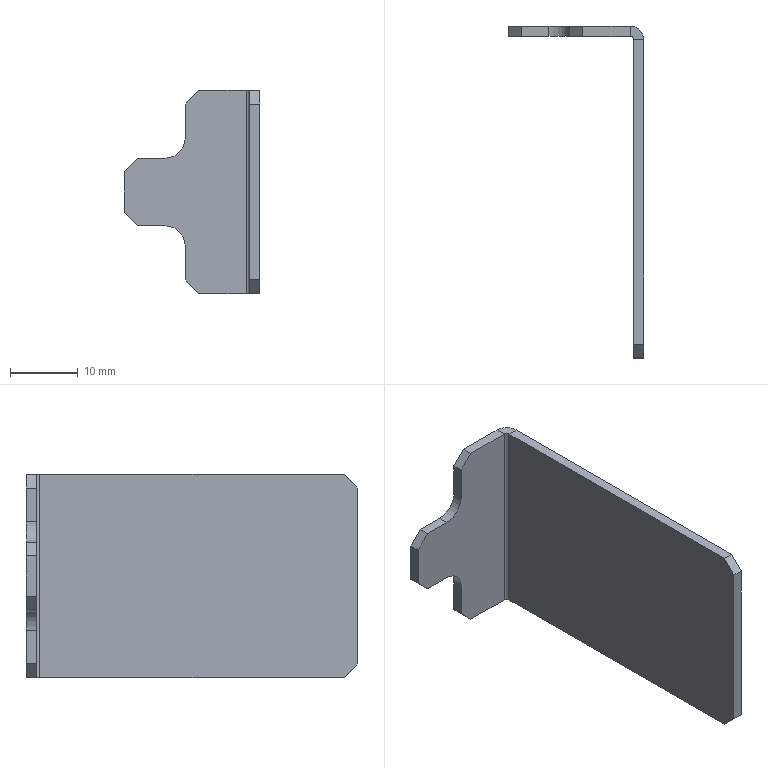Part | SolidWorks | features Chamfer 2, Cut 2, Fillet 1, FlatPattern 1, SMBaseFlange 1, SheetMetal 1 | 1 solid | 26 faces | box 20 x 49 x 30 mm | volume 2731 mm3 | plane 22 | cylinder 4 | commonest cylinder face diameters 6 x2 1 x1 4 x1
STEP:
#1=CARTESIAN_POINT('',(0.,-2.,15.));
#2=VERTEX_POINT('',#1);
#3=CARTESIAN_POINT('',(-1.5,-2.,15.));
#4=VERTEX_POINT('',#3);
#5=CARTESIAN_POINT('',(0.,-2.,15.));
#6=DIRECTION('',(-1.,0.,0.));
#7=VECTOR('',#6,1000.);
#8=LINE('',#5,#7);
#9=EDGE_CURVE('',#2,#4,#8,.T.);
#10=ORIENTED_EDGE('',*,*,#9,.F.);
#11=CARTESIAN_POINT('',(-2.,0.,15.));
#12=VERTEX_POINT('',#11);
#13=CARTESIAN_POINT('',(-2.,-2.,15.));
#14=DIRECTION('',(0.,0.,-1.));
#15=DIRECTION('',(1.,0.,0.));
#16=AXIS2_PLACEMENT_3D('',#13,#14,#15);
#17=CIRCLE('',#16,2.);
#18=EDGE_CURVE('',#12,#2,#17,.T.);
#19=ORIENTED_EDGE('',*,*,#18,.F.);
#20=CARTESIAN_POINT('',(-2.,-1.5,15.));
#21=VERTEX_POINT('',#20);
#22=CARTESIAN_POINT('',(-2.,-1.5,15.));
#23=DIRECTION('',(0.,1.,0.));
#24=VECTOR('',#23,1000.);
#25=LINE('',#22,#24);
#26=EDGE_CURVE('',#21,#12,#25,.T.);
#27=ORIENTED_EDGE('',*,*,#26,.F.);
#28=CARTESIAN_POINT('',(-2.,-2.,15.));
#29=DIRECTION('',(0.,0.,-1.));
#30=DIRECTION('',(1.,0.,0.));
#31=AXIS2_PLACEMENT_3D('',#28,#29,#30);
#32=CIRCLE('',#31,0.5);
#33=EDGE_CURVE('',#21,#4,#32,.T.);
#34=ORIENTED_EDGE('',*,*,#33,.T.);
#35=EDGE_LOOP('',(#10,#19,#27,#34));
#36=FACE_OUTER_BOUND('',#35,.T.);
#37=CARTESIAN_POINT('',(0.,-2.,15.));
#38=DIRECTION('',(0.,0.,1.));
#39=DIRECTION('',(1.,0.,0.));
#40=AXIS2_PLACEMENT_3D('',#37,#38,#39);
#41=PLANE('',#40);
#42=ADVANCED_FACE('',(#36),#41,.T.);
#43=CARTESIAN_POINT('',(-1.5,-47.,15.));
#44=VERTEX_POINT('',#43);
#45=CARTESIAN_POINT('',(-1.5,0.,15.));
#46=DIRECTION('',(0.,-1.,0.));
#47=VECTOR('',#46,1000.);
#48=LINE('',#45,#47);
#49=EDGE_CURVE('',#4,#44,#48,.T.);
#50=ORIENTED_EDGE('',*,*,#49,.T.);
#51=CARTESIAN_POINT('',(0.,-47.,15.));
#52=VERTEX_POINT('',#51);
#53=CARTESIAN_POINT('',(-2.,-47.,15.));
#54=DIRECTION('',(1.,0.,0.));
#55=VECTOR('',#54,1000.);
#56=LINE('',#53,#55);
#57=EDGE_CURVE('',#44,#52,#56,.T.);
#58=ORIENTED_EDGE('',*,*,#57,.T.);
#59=CARTESIAN_POINT('',(0.,0.,15.));
#60=DIRECTION('',(0.,-1.,0.));
#61=VECTOR('',#60,1000.);
#62=LINE('',#59,#61);
#63=EDGE_CURVE('',#2,#52,#62,.T.);
#64=ORIENTED_EDGE('',*,*,#63,.F.);
#65=ORIENTED_EDGE('',*,*,#9,.T.);
#66=EDGE_LOOP('',(#50,#58,#64,#65));
#67=FACE_OUTER_BOUND('',#66,.T.);
#68=CARTESIAN_POINT('',(-2.,-1.5,15.));
#69=DIRECTION('',(0.,0.,1.));
#70=DIRECTION('',(1.,0.,0.));
#71=AXIS2_PLACEMENT_3D('',#68,#69,#70);
#72=PLANE('',#71);
#73=ADVANCED_FACE('',(#67),#72,.T.);
#74=CARTESIAN_POINT('',(-2.,0.,-15.));
#75=VERTEX_POINT('',#74);
#76=CARTESIAN_POINT('',(-2.,-1.5,-15.));
#77=VERTEX_POINT('',#76);
#78=CARTESIAN_POINT('',(-2.,0.,-15.));
#79=DIRECTION('',(0.,-1.,0.));
#80=VECTOR('',#79,1000.);
#81=LINE('',#78,#80);
#82=EDGE_CURVE('',#75,#77,#81,.T.);
#83=ORIENTED_EDGE('',*,*,#82,.F.);
#84=CARTESIAN_POINT('',(0.,-2.,-15.));
#85=VERTEX_POINT('',#84);
#86=CARTESIAN_POINT('',(-2.,-2.,-15.));
#87=DIRECTION('',(0.,0.,-1.));
#88=DIRECTION('',(1.,0.,0.));
#89=AXIS2_PLACEMENT_3D('',#86,#87,#88);
#90=CIRCLE('',#89,2.);
#91=EDGE_CURVE('',#75,#85,#90,.T.);
#92=ORIENTED_EDGE('',*,*,#91,.T.);
#93=CARTESIAN_POINT('',(-1.5,-2.,-15.));
#94=VERTEX_POINT('',#93);
#95=CARTESIAN_POINT('',(-1.5,-2.,-15.));
#96=DIRECTION('',(1.,0.,0.));
#97=VECTOR('',#96,1000.);
#98=LINE('',#95,#97);
#99=EDGE_CURVE('',#94,#85,#98,.T.);
#100=ORIENTED_EDGE('',*,*,#99,.F.);
#101=CARTESIAN_POINT('',(-2.,-2.,-15.));
#102=DIRECTION('',(0.,0.,-1.));
#103=DIRECTION('',(1.,0.,0.));
#104=AXIS2_PLACEMENT_3D('',#101,#102,#103);
#105=CIRCLE('',#104,0.5);
#106=EDGE_CURVE('',#77,#94,#105,.T.);
#107=ORIENTED_EDGE('',*,*,#106,.F.);
#108=EDGE_LOOP('',(#83,#92,#100,#107));
#109=FACE_OUTER_BOUND('',#108,.T.);
#110=CARTESIAN_POINT('',(-2.,0.,-15.));
#111=DIRECTION('',(0.,0.,-1.));
#112=DIRECTION('',(-1.,0.,0.));
#113=AXIS2_PLACEMENT_3D('',#110,#111,#112);
#114=PLANE('',#113);
#115=ADVANCED_FACE('',(#109),#114,.T.);
#116=CARTESIAN_POINT('',(-9.,-1.5,-15.));
#117=VERTEX_POINT('',#116);
#118=CARTESIAN_POINT('',(-20.,-1.5,-15.));
#119=DIRECTION('',(1.,0.,0.));
#120=VECTOR('',#119,1000.);
#121=LINE('',#118,#120);
#122=EDGE_CURVE('',#117,#77,#121,.T.);
#123=ORIENTED_EDGE('',*,*,#122,.F.);
#124=CARTESIAN_POINT('',(-9.,0.,-15.));
#125=VERTEX_POINT('',#124);
#126=CARTESIAN_POINT('',(-9.,0.,-15.));
#127=DIRECTION('',(0.,1.,0.));
#128=VECTOR('',#127,1000.);
#129=LINE('',#126,#128);
#130=EDGE_CURVE('',#117,#125,#129,.T.);
#131=ORIENTED_EDGE('',*,*,#130,.T.);
#132=CARTESIAN_POINT('',(-20.,0.,-15.));
#133=DIRECTION('',(1.,0.,0.));
#134=VECTOR('',#133,1000.);
#135=LINE('',#132,#134);
#136=EDGE_CURVE('',#125,#75,#135,.T.);
#137=ORIENTED_EDGE('',*,*,#136,.T.);
#138=ORIENTED_EDGE('',*,*,#82,.T.);
#139=EDGE_LOOP('',(#123,#131,#137,#138));
#140=FACE_OUTER_BOUND('',#139,.T.);
#141=CARTESIAN_POINT('',(-1.5,-2.,-15.));
#142=DIRECTION('',(0.,0.,-1.));
#143=DIRECTION('',(-1.,0.,0.));
#144=AXIS2_PLACEMENT_3D('',#141,#142,#143);
#145=PLANE('',#144);
#146=ADVANCED_FACE('',(#140),#145,.T.);
#147=CARTESIAN_POINT('',(-1.5,-47.,-15.));
#148=VERTEX_POINT('',#147);
#149=CARTESIAN_POINT('',(-1.5,0.,-15.));
#150=DIRECTION('',(0.,-1.,0.));
#151=VECTOR('',#150,1000.);
#152=LINE('',#149,#151);
#153=EDGE_CURVE('',#94,#148,#152,.T.);
#154=ORIENTED_EDGE('',*,*,#153,.T.);
#155=CARTESIAN_POINT('',(-1.5,-49.,-13.));
#156=VERTEX_POINT('',#155);
#157=CARTESIAN_POINT('',(-1.5,-47.,-15.));
#158=DIRECTION('',(0.,-0.7071,0.7071));
#159=VECTOR('',#158,1000.);
#160=LINE('',#157,#159);
#161=EDGE_CURVE('',#148,#156,#160,.T.);
#162=ORIENTED_EDGE('',*,*,#161,.T.);
#163=CARTESIAN_POINT('',(-1.5,-49.,13.));
#164=VERTEX_POINT('',#163);
#165=CARTESIAN_POINT('',(-1.5,-49.,15.));
#166=DIRECTION('',(0.,0.,-1.));
#167=VECTOR('',#166,1000.);
#168=LINE('',#165,#167);
#169=EDGE_CURVE('',#164,#156,#168,.T.);
#170=ORIENTED_EDGE('',*,*,#169,.F.);
#171=CARTESIAN_POINT('',(-1.5,-49.,13.));
#172=DIRECTION('',(0.,0.7071,0.7071));
#173=VECTOR('',#172,1000.);
#174=LINE('',#171,#173);
#175=EDGE_CURVE('',#164,#44,#174,.T.);
#176=ORIENTED_EDGE('',*,*,#175,.T.);
#177=ORIENTED_EDGE('',*,*,#49,.F.);
#178=CARTESIAN_POINT('',(-1.5,-2.,15.));
#179=DIRECTION('',(0.,0.,-1.));
#180=VECTOR('',#179,1000.);
#181=LINE('',#178,#180);
#182=EDGE_CURVE('',#4,#94,#181,.T.);
#183=ORIENTED_EDGE('',*,*,#182,.T.);
#184=EDGE_LOOP('',(#154,#162,#170,#176,#177,#183));
#185=FACE_OUTER_BOUND('',#184,.T.);
#186=CARTESIAN_POINT('',(-1.5,0.,15.));
#187=DIRECTION('',(1.,0.,0.));
#188=DIRECTION('',(0.,1.,0.));
#189=AXIS2_PLACEMENT_3D('',#186,#187,#188);
#190=PLANE('',#189);
#191=ADVANCED_FACE('',(#185),#190,.F.);
#192=ORIENTED_EDGE('',*,*,#169,.T.);
#193=CARTESIAN_POINT('',(0.,-49.,-13.));
#194=VERTEX_POINT('',#193);
#195=CARTESIAN_POINT('',(0.,-49.,-13.));
#196=DIRECTION('',(1.,0.,0.));
#197=VECTOR('',#196,1000.);
#198=LINE('',#195,#197);
#199=EDGE_CURVE('',#156,#194,#198,.T.);
#200=ORIENTED_EDGE('',*,*,#199,.T.);
#201=CARTESIAN_POINT('',(0.,-49.,13.));
#202=VERTEX_POINT('',#201);
#203=CARTESIAN_POINT('',(0.,-49.,15.));
#204=DIRECTION('',(0.,0.,-1.));
#205=VECTOR('',#204,1000.);
#206=LINE('',#203,#205);
#207=EDGE_CURVE('',#202,#194,#206,.T.);
#208=ORIENTED_EDGE('',*,*,#207,.F.);
#209=CARTESIAN_POINT('',(0.,-49.,13.));
#210=DIRECTION('',(-1.,0.,0.));
#211=VECTOR('',#210,1000.);
#212=LINE('',#209,#211);
#213=EDGE_CURVE('',#202,#164,#212,.T.);
#214=ORIENTED_EDGE('',*,*,#213,.T.);
#215=EDGE_LOOP('',(#192,#200,#208,#214));
#216=FACE_OUTER_BOUND('',#215,.T.);
#217=CARTESIAN_POINT('',(0.,-49.,15.));
#218=DIRECTION('',(0.,-1.,0.));
#219=DIRECTION('',(0.,0.,-1.));
#220=AXIS2_PLACEMENT_3D('',#217,#218,#219);
#221=PLANE('',#220);
#222=ADVANCED_FACE('',(#216),#221,.T.);
#223=ORIENTED_EDGE('',*,*,#207,.T.);
#224=CARTESIAN_POINT('',(0.,-47.,-15.));
#225=VERTEX_POINT('',#224);
#226=CARTESIAN_POINT('',(0.,-38.5,-23.5));
#227=DIRECTION('',(0.,0.7071,-0.7071));
#228=VECTOR('',#227,1000.);
#229=LINE('',#226,#228);
#230=EDGE_CURVE('',#194,#225,#229,.T.);
#231=ORIENTED_EDGE('',*,*,#230,.T.);
#232=CARTESIAN_POINT('',(0.,0.,-15.));
#233=DIRECTION('',(0.,-1.,0.));
#234=VECTOR('',#233,1000.);
#235=LINE('',#232,#234);
#236=EDGE_CURVE('',#85,#225,#235,.T.);
#237=ORIENTED_EDGE('',*,*,#236,.F.);
#238=CARTESIAN_POINT('',(0.,-2.,15.));
#239=DIRECTION('',(0.,0.,-1.));
#240=VECTOR('',#239,1000.);
#241=LINE('',#238,#240);
#242=EDGE_CURVE('',#2,#85,#241,.T.);
#243=ORIENTED_EDGE('',*,*,#242,.F.);
#244=ORIENTED_EDGE('',*,*,#63,.T.);
#245=CARTESIAN_POINT('',(0.,-23.5,38.5));
#246=DIRECTION('',(0.,-0.7071,-0.7071));
#247=VECTOR('',#246,1000.);
#248=LINE('',#245,#247);
#249=EDGE_CURVE('',#52,#202,#248,.T.);
#250=ORIENTED_EDGE('',*,*,#249,.T.);
#251=EDGE_LOOP('',(#223,#231,#237,#243,#244,#250));
#252=FACE_OUTER_BOUND('',#251,.T.);
#253=CARTESIAN_POINT('',(0.,0.,15.));
#254=DIRECTION('',(1.,0.,0.));
#255=DIRECTION('',(0.,1.,0.));
#256=AXIS2_PLACEMENT_3D('',#253,#254,#255);
#257=PLANE('',#256);
#258=ADVANCED_FACE('',(#252),#257,.T.);
#259=ORIENTED_EDGE('',*,*,#91,.F.);
#260=CARTESIAN_POINT('',(-2.,0.,15.));
#261=DIRECTION('',(0.,0.,-1.));
#262=VECTOR('',#261,1000.);
#263=LINE('',#260,#262);
#264=EDGE_CURVE('',#12,#75,#263,.T.);
#265=ORIENTED_EDGE('',*,*,#264,.F.);
#266=ORIENTED_EDGE('',*,*,#18,.T.);
#267=ORIENTED_EDGE('',*,*,#242,.T.);
#268=EDGE_LOOP('',(#259,#265,#266,#267));
#269=FACE_OUTER_BOUND('',#268,.T.);
#270=CARTESIAN_POINT('',(-2.,-2.,15.));
#271=DIRECTION('',(0.,0.,-1.));
#272=DIRECTION('',(-1.,0.,0.));
#273=AXIS2_PLACEMENT_3D('',#270,#271,#272);
#274=CYLINDRICAL_SURFACE('',#273,2.);
#275=ADVANCED_FACE('',(#269),#274,.T.);
#276=ORIENTED_EDGE('',*,*,#136,.F.);
#277=CARTESIAN_POINT('',(-11.,0.,-13.));
#278=VERTEX_POINT('',#277);
#279=CARTESIAN_POINT('',(-29.5,0.,5.5));
#280=DIRECTION('',(-0.7071,0.,0.7071));
#281=VECTOR('',#280,1000.);
#282=LINE('',#279,#281);
#283=EDGE_CURVE('',#125,#278,#282,.T.);
#284=ORIENTED_EDGE('',*,*,#283,.T.);
#285=CARTESIAN_POINT('',(-11.,0.,-8.));
#286=VERTEX_POINT('',#285);
#287=CARTESIAN_POINT('',(-11.,0.,-15.));
#288=DIRECTION('',(0.,0.,1.));
#289=VECTOR('',#288,1000.);
#290=LINE('',#287,#289);
#291=EDGE_CURVE('',#278,#286,#290,.T.);
#292=ORIENTED_EDGE('',*,*,#291,.T.);
#293=CARTESIAN_POINT('',(-14.,0.,-5.));
#294=VERTEX_POINT('',#293);
#295=CARTESIAN_POINT('',(-14.,0.,-8.));
#296=DIRECTION('',(0.,-1.,0.));
#297=DIRECTION('',(0.,0.,1.));
#298=AXIS2_PLACEMENT_3D('',#295,#296,#297);
#299=CIRCLE('',#298,3.);
#300=EDGE_CURVE('',#286,#294,#299,.T.);
#301=ORIENTED_EDGE('',*,*,#300,.T.);
#302=CARTESIAN_POINT('',(-18.,0.,-5.));
#303=VERTEX_POINT('',#302);
#304=CARTESIAN_POINT('',(-20.,0.,-5.));
#305=DIRECTION('',(-1.,0.,0.));
#306=VECTOR('',#305,1000.);
#307=LINE('',#304,#306);
#308=EDGE_CURVE('',#294,#303,#307,.T.);
#309=ORIENTED_EDGE('',*,*,#308,.T.);
#310=CARTESIAN_POINT('',(-20.,0.,-3.));
#311=VERTEX_POINT('',#310);
#312=CARTESIAN_POINT('',(-29.,0.,6.));
#313=DIRECTION('',(-0.7071,0.,0.7071));
#314=VECTOR('',#313,1000.);
#315=LINE('',#312,#314);
#316=EDGE_CURVE('',#303,#311,#315,.T.);
#317=ORIENTED_EDGE('',*,*,#316,.T.);
#318=CARTESIAN_POINT('',(-20.,0.,3.));
#319=VERTEX_POINT('',#318);
#320=CARTESIAN_POINT('',(-20.,0.,15.));
#321=DIRECTION('',(0.,0.,-1.));
#322=VECTOR('',#321,1000.);
#323=LINE('',#320,#322);
#324=EDGE_CURVE('',#319,#311,#323,.T.);
#325=ORIENTED_EDGE('',*,*,#324,.F.);
#326=CARTESIAN_POINT('',(-18.,0.,5.));
#327=VERTEX_POINT('',#326);
#328=CARTESIAN_POINT('',(-14.,0.,9.));
#329=DIRECTION('',(0.7071,0.,0.7071));
#330=VECTOR('',#329,1000.);
#331=LINE('',#328,#330);
#332=EDGE_CURVE('',#319,#327,#331,.T.);
#333=ORIENTED_EDGE('',*,*,#332,.T.);
#334=CARTESIAN_POINT('',(-14.,0.,5.));
#335=VERTEX_POINT('',#334);
#336=CARTESIAN_POINT('',(-11.,0.,5.));
#337=DIRECTION('',(1.,0.,0.));
#338=VECTOR('',#337,1000.);
#339=LINE('',#336,#338);
#340=EDGE_CURVE('',#327,#335,#339,.T.);
#341=ORIENTED_EDGE('',*,*,#340,.T.);
#342=CARTESIAN_POINT('',(-11.,0.,8.));
#343=VERTEX_POINT('',#342);
#344=CARTESIAN_POINT('',(-14.,0.,8.));
#345=DIRECTION('',(0.,-1.,0.));
#346=DIRECTION('',(0.,0.,1.));
#347=AXIS2_PLACEMENT_3D('',#344,#345,#346);
#348=CIRCLE('',#347,3.);
#349=EDGE_CURVE('',#335,#343,#348,.T.);
#350=ORIENTED_EDGE('',*,*,#349,.T.);
#351=CARTESIAN_POINT('',(-11.,0.,13.));
#352=VERTEX_POINT('',#351);
#353=CARTESIAN_POINT('',(-11.,0.,15.));
#354=DIRECTION('',(0.,0.,1.));
#355=VECTOR('',#354,1000.);
#356=LINE('',#353,#355);
#357=EDGE_CURVE('',#343,#352,#356,.T.);
#358=ORIENTED_EDGE('',*,*,#357,.T.);
#359=CARTESIAN_POINT('',(-9.,0.,15.));
#360=VERTEX_POINT('',#359);
#361=CARTESIAN_POINT('',(-14.5,0.,9.5));
#362=DIRECTION('',(0.7071,0.,0.7071));
#363=VECTOR('',#362,1000.);
#364=LINE('',#361,#363);
#365=EDGE_CURVE('',#352,#360,#364,.T.);
#366=ORIENTED_EDGE('',*,*,#365,.T.);
#367=CARTESIAN_POINT('',(-20.,0.,15.));
#368=DIRECTION('',(1.,0.,0.));
#369=VECTOR('',#368,1000.);
#370=LINE('',#367,#369);
#371=EDGE_CURVE('',#360,#12,#370,.T.);
#372=ORIENTED_EDGE('',*,*,#371,.T.);
#373=ORIENTED_EDGE('',*,*,#264,.T.);
#374=EDGE_LOOP('',(#276,#284,#292,#301,#309,#317,#325,#333,#341,#350,#358,#366,#372,#373));
#375=FACE_OUTER_BOUND('',#374,.T.);
#376=CARTESIAN_POINT('',(-20.,0.,15.));
#377=DIRECTION('',(0.,1.,0.));
#378=DIRECTION('',(0.,0.,1.));
#379=AXIS2_PLACEMENT_3D('',#376,#377,#378);
#380=PLANE('',#379);
#381=ADVANCED_FACE('',(#375),#380,.T.);
#382=CARTESIAN_POINT('',(-20.,-1.5,3.));
#383=VERTEX_POINT('',#382);
#384=CARTESIAN_POINT('',(-20.,-1.5,-3.));
#385=VERTEX_POINT('',#384);
#386=CARTESIAN_POINT('',(-20.,-1.5,15.));
#387=DIRECTION('',(0.,0.,-1.));
#388=VECTOR('',#387,1000.);
#389=LINE('',#386,#388);
#390=EDGE_CURVE('',#383,#385,#389,.T.);
#391=ORIENTED_EDGE('',*,*,#390,.F.);
#392=CARTESIAN_POINT('',(-20.,0.,3.));
#393=DIRECTION('',(0.,1.,0.));
#394=VECTOR('',#393,1000.);
#395=LINE('',#392,#394);
#396=EDGE_CURVE('',#383,#319,#395,.T.);
#397=ORIENTED_EDGE('',*,*,#396,.T.);
#398=ORIENTED_EDGE('',*,*,#324,.T.);
#399=CARTESIAN_POINT('',(-20.,-1.5,-3.));
#400=DIRECTION('',(0.,-1.,0.));
#401=VECTOR('',#400,1000.);
#402=LINE('',#399,#401);
#403=EDGE_CURVE('',#311,#385,#402,.T.);
#404=ORIENTED_EDGE('',*,*,#403,.T.);
#405=EDGE_LOOP('',(#391,#397,#398,#404));
#406=FACE_OUTER_BOUND('',#405,.T.);
#407=CARTESIAN_POINT('',(-20.,-1.5,15.));
#408=DIRECTION('',(-1.,0.,0.));
#409=DIRECTION('',(0.,0.,1.));
#410=AXIS2_PLACEMENT_3D('',#407,#408,#409);
#411=PLANE('',#410);
#412=ADVANCED_FACE('',(#406),#411,.T.);
#413=CARTESIAN_POINT('',(-11.,-1.5,-13.));
#414=VERTEX_POINT('',#413);
#415=CARTESIAN_POINT('',(-11.,-1.5,-8.));
#416=VERTEX_POINT('',#415);
#417=CARTESIAN_POINT('',(-11.,-1.5,-15.));
#418=DIRECTION('',(0.,0.,1.));
#419=VECTOR('',#418,1000.);
#420=LINE('',#417,#419);
#421=EDGE_CURVE('',#414,#416,#420,.T.);
#422=ORIENTED_EDGE('',*,*,#421,.F.);
#423=CARTESIAN_POINT('',(-11.,-1.5,-13.));
#424=DIRECTION('',(0.7071,0.,-0.7071));
#425=VECTOR('',#424,1000.);
#426=LINE('',#423,#425);
#427=EDGE_CURVE('',#414,#117,#426,.T.);
#428=ORIENTED_EDGE('',*,*,#427,.T.);
#429=ORIENTED_EDGE('',*,*,#122,.T.);
#430=CARTESIAN_POINT('',(-2.,-1.5,15.));
#431=DIRECTION('',(0.,0.,-1.));
#432=VECTOR('',#431,1000.);
#433=LINE('',#430,#432);
#434=EDGE_CURVE('',#21,#77,#433,.T.);
#435=ORIENTED_EDGE('',*,*,#434,.F.);
#436=CARTESIAN_POINT('',(-9.,-1.5,15.));
#437=VERTEX_POINT('',#436);
#438=CARTESIAN_POINT('',(-20.,-1.5,15.));
#439=DIRECTION('',(1.,0.,0.));
#440=VECTOR('',#439,1000.);
#441=LINE('',#438,#440);
#442=EDGE_CURVE('',#437,#21,#441,.T.);
#443=ORIENTED_EDGE('',*,*,#442,.F.);
#444=CARTESIAN_POINT('',(-11.,-1.5,13.));
#445=VERTEX_POINT('',#444);
#446=CARTESIAN_POINT('',(-9.,-1.5,15.));
#447=DIRECTION('',(-0.7071,0.,-0.7071));
#448=VECTOR('',#447,1000.);
#449=LINE('',#446,#448);
#450=EDGE_CURVE('',#437,#445,#449,.T.);
#451=ORIENTED_EDGE('',*,*,#450,.T.);
#452=CARTESIAN_POINT('',(-11.,-1.5,8.));
#453=VERTEX_POINT('',#452);
#454=CARTESIAN_POINT('',(-11.,-1.5,15.));
#455=DIRECTION('',(0.,0.,1.));
#456=VECTOR('',#455,1000.);
#457=LINE('',#454,#456);
#458=EDGE_CURVE('',#453,#445,#457,.T.);
#459=ORIENTED_EDGE('',*,*,#458,.F.);
#460=CARTESIAN_POINT('',(-14.,-1.5,5.));
#461=VERTEX_POINT('',#460);
#462=CARTESIAN_POINT('',(-14.,-1.5,8.));
#463=DIRECTION('',(0.,1.,0.));
#464=DIRECTION('',(0.,0.,1.));
#465=AXIS2_PLACEMENT_3D('',#462,#463,#464);
#466=CIRCLE('',#465,3.);
#467=EDGE_CURVE('',#453,#461,#466,.T.);
#468=ORIENTED_EDGE('',*,*,#467,.T.);
#469=CARTESIAN_POINT('',(-18.,-1.5,5.));
#470=VERTEX_POINT('',#469);
#471=CARTESIAN_POINT('',(-11.,-1.5,5.));
#472=DIRECTION('',(1.,0.,0.));
#473=VECTOR('',#472,1000.);
#474=LINE('',#471,#473);
#475=EDGE_CURVE('',#470,#461,#474,.T.);
#476=ORIENTED_EDGE('',*,*,#475,.F.);
#477=CARTESIAN_POINT('',(-18.,-1.5,5.));
#478=DIRECTION('',(-0.7071,0.,-0.7071));
#479=VECTOR('',#478,1000.);
#480=LINE('',#477,#479);
#481=EDGE_CURVE('',#470,#383,#480,.T.);
#482=ORIENTED_EDGE('',*,*,#481,.T.);
#483=ORIENTED_EDGE('',*,*,#390,.T.);
#484=CARTESIAN_POINT('',(-18.,-1.5,-5.));
#485=VERTEX_POINT('',#484);
#486=CARTESIAN_POINT('',(-20.,-1.5,-3.));
#487=DIRECTION('',(0.7071,0.,-0.7071));
#488=VECTOR('',#487,1000.);
#489=LINE('',#486,#488);
#490=EDGE_CURVE('',#385,#485,#489,.T.);
#491=ORIENTED_EDGE('',*,*,#490,.T.);
#492=CARTESIAN_POINT('',(-14.,-1.5,-5.));
#493=VERTEX_POINT('',#492);
#494=CARTESIAN_POINT('',(-20.,-1.5,-5.));
#495=DIRECTION('',(-1.,0.,0.));
#496=VECTOR('',#495,1000.);
#497=LINE('',#494,#496);
#498=EDGE_CURVE('',#493,#485,#497,.T.);
#499=ORIENTED_EDGE('',*,*,#498,.F.);
#500=CARTESIAN_POINT('',(-14.,-1.5,-8.));
#501=DIRECTION('',(0.,1.,0.));
#502=DIRECTION('',(0.,0.,1.));
#503=AXIS2_PLACEMENT_3D('',#500,#501,#502);
#504=CIRCLE('',#503,3.);
#505=EDGE_CURVE('',#493,#416,#504,.T.);
#506=ORIENTED_EDGE('',*,*,#505,.T.);
#507=EDGE_LOOP('',(#422,#428,#429,#435,#443,#451,#459,#468,#476,#482,#483,#491,#499,#506));
#508=FACE_OUTER_BOUND('',#507,.T.);
#509=CARTESIAN_POINT('',(-20.,-1.5,15.));
#510=DIRECTION('',(0.,1.,0.));
#511=DIRECTION('',(0.,0.,1.));
#512=AXIS2_PLACEMENT_3D('',#509,#510,#511);
#513=PLANE('',#512);
#514=ADVANCED_FACE('',(#508),#513,.F.);
#515=ORIENTED_EDGE('',*,*,#106,.T.);
#516=ORIENTED_EDGE('',*,*,#182,.F.);
#517=ORIENTED_EDGE('',*,*,#33,.F.);
#518=ORIENTED_EDGE('',*,*,#434,.T.);
#519=EDGE_LOOP('',(#515,#516,#517,#518));
#520=FACE_OUTER_BOUND('',#519,.T.);
#521=CARTESIAN_POINT('',(-2.,-2.,15.));
#522=DIRECTION('',(0.,0.,-1.));
#523=DIRECTION('',(-1.,0.,0.));
#524=AXIS2_PLACEMENT_3D('',#521,#522,#523);
#525=CYLINDRICAL_SURFACE('',#524,0.5);
#526=ADVANCED_FACE('',(#520),#525,.F.);
#527=ORIENTED_EDGE('',*,*,#371,.F.);
#528=CARTESIAN_POINT('',(-9.,-1.5,15.));
#529=DIRECTION('',(0.,-1.,0.));
#530=VECTOR('',#529,1000.);
#531=LINE('',#528,#530);
#532=EDGE_CURVE('',#360,#437,#531,.T.);
#533=ORIENTED_EDGE('',*,*,#532,.T.);
#534=ORIENTED_EDGE('',*,*,#442,.T.);
#535=ORIENTED_EDGE('',*,*,#26,.T.);
#536=EDGE_LOOP('',(#527,#533,#534,#535));
#537=FACE_OUTER_BOUND('',#536,.T.);
#538=CARTESIAN_POINT('',(-2.,-2.,15.));
#539=DIRECTION('',(0.,0.,1.));
#540=DIRECTION('',(1.,0.,0.));
#541=AXIS2_PLACEMENT_3D('',#538,#539,#540);
#542=PLANE('',#541);
#543=ADVANCED_FACE('',(#537),#542,.T.);
#544=ORIENTED_EDGE('',*,*,#236,.T.);
#545=CARTESIAN_POINT('',(-1.5,-47.,-15.));
#546=DIRECTION('',(-1.,0.,0.));
#547=VECTOR('',#546,1000.);
#548=LINE('',#545,#547);
#549=EDGE_CURVE('',#225,#148,#548,.T.);
#550=ORIENTED_EDGE('',*,*,#549,.T.);
#551=ORIENTED_EDGE('',*,*,#153,.F.);
#552=ORIENTED_EDGE('',*,*,#99,.T.);
#553=EDGE_LOOP('',(#544,#550,#551,#552));
#554=FACE_OUTER_BOUND('',#553,.T.);
#555=CARTESIAN_POINT('',(-2.,-2.,-15.));
#556=DIRECTION('',(0.,0.,1.));
#557=DIRECTION('',(1.,0.,0.));
#558=AXIS2_PLACEMENT_3D('',#555,#556,#557);
#559=PLANE('',#558);
#560=ADVANCED_FACE('',(#554),#559,.F.);
#561=ORIENTED_EDGE('',*,*,#458,.T.);
#562=CARTESIAN_POINT('',(-11.,0.,13.));
#563=DIRECTION('',(0.,1.,0.));
#564=VECTOR('',#563,1000.);
#565=LINE('',#562,#564);
#566=EDGE_CURVE('',#445,#352,#565,.T.);
#567=ORIENTED_EDGE('',*,*,#566,.T.);
#568=ORIENTED_EDGE('',*,*,#357,.F.);
#569=CARTESIAN_POINT('',(-11.,-1.5,8.));
#570=DIRECTION('',(0.,-1.,0.));
#571=VECTOR('',#570,1000.);
#572=LINE('',#569,#571);
#573=EDGE_CURVE('',#343,#453,#572,.T.);
#574=ORIENTED_EDGE('',*,*,#573,.T.);
#575=EDGE_LOOP('',(#561,#567,#568,#574));
#576=FACE_OUTER_BOUND('',#575,.T.);
#577=CARTESIAN_POINT('',(-11.,0.,15.));
#578=DIRECTION('',(1.,0.,0.));
#579=DIRECTION('',(0.,0.,-1.));
#580=AXIS2_PLACEMENT_3D('',#577,#578,#579);
#581=PLANE('',#580);
#582=ADVANCED_FACE('',(#576),#581,.F.);
#583=ORIENTED_EDGE('',*,*,#340,.F.);
#584=CARTESIAN_POINT('',(-18.,-1.5,5.));
#585=DIRECTION('',(0.,-1.,0.));
#586=VECTOR('',#585,1000.);
#587=LINE('',#584,#586);
#588=EDGE_CURVE('',#327,#470,#587,.T.);
#589=ORIENTED_EDGE('',*,*,#588,.T.);
#590=ORIENTED_EDGE('',*,*,#475,.T.);
#591=CARTESIAN_POINT('',(-14.,0.,5.));
#592=DIRECTION('',(0.,1.,0.));
#593=VECTOR('',#592,1000.);
#594=LINE('',#591,#593);
#595=EDGE_CURVE('',#461,#335,#594,.T.);
#596=ORIENTED_EDGE('',*,*,#595,.T.);
#597=EDGE_LOOP('',(#583,#589,#590,#596));
#598=FACE_OUTER_BOUND('',#597,.T.);
#599=CARTESIAN_POINT('',(-11.,0.,5.));
#600=DIRECTION('',(0.,0.,-1.));
#601=DIRECTION('',(-1.,0.,0.));
#602=AXIS2_PLACEMENT_3D('',#599,#600,#601);
#603=PLANE('',#602);
#604=ADVANCED_FACE('',(#598),#603,.F.);
#605=ORIENTED_EDGE('',*,*,#498,.T.);
#606=CARTESIAN_POINT('',(-18.,0.,-5.));
#607=DIRECTION('',(0.,1.,0.));
#608=VECTOR('',#607,1000.);
#609=LINE('',#606,#608);
#610=EDGE_CURVE('',#485,#303,#609,.T.);
#611=ORIENTED_EDGE('',*,*,#610,.T.);
#612=ORIENTED_EDGE('',*,*,#308,.F.);
#613=CARTESIAN_POINT('',(-14.,-1.5,-5.));
#614=DIRECTION('',(0.,-1.,0.));
#615=VECTOR('',#614,1000.);
#616=LINE('',#613,#615);
#617=EDGE_CURVE('',#294,#493,#616,.T.);
#618=ORIENTED_EDGE('',*,*,#617,.T.);
#619=EDGE_LOOP('',(#605,#611,#612,#618));
#620=FACE_OUTER_BOUND('',#619,.T.);
#621=CARTESIAN_POINT('',(-20.,0.,-5.));
#622=DIRECTION('',(0.,0.,1.));
#623=DIRECTION('',(1.,0.,0.));
#624=AXIS2_PLACEMENT_3D('',#621,#622,#623);
#625=PLANE('',#624);
#626=ADVANCED_FACE('',(#620),#625,.F.);
#627=ORIENTED_EDGE('',*,*,#291,.F.);
#628=CARTESIAN_POINT('',(-11.,-1.5,-13.));
#629=DIRECTION('',(0.,-1.,0.));
#630=VECTOR('',#629,1000.);
#631=LINE('',#628,#630);
#632=EDGE_CURVE('',#278,#414,#631,.T.);
#633=ORIENTED_EDGE('',*,*,#632,.T.);
#634=ORIENTED_EDGE('',*,*,#421,.T.);
#635=CARTESIAN_POINT('',(-11.,0.,-8.));
#636=DIRECTION('',(0.,1.,0.));
#637=VECTOR('',#636,1000.);
#638=LINE('',#635,#637);
#639=EDGE_CURVE('',#416,#286,#638,.T.);
#640=ORIENTED_EDGE('',*,*,#639,.T.);
#641=EDGE_LOOP('',(#627,#633,#634,#640));
#642=FACE_OUTER_BOUND('',#641,.T.);
#643=CARTESIAN_POINT('',(-11.,0.,-15.));
#644=DIRECTION('',(1.,0.,0.));
#645=DIRECTION('',(0.,0.,-1.));
#646=AXIS2_PLACEMENT_3D('',#643,#644,#645);
#647=PLANE('',#646);
#648=ADVANCED_FACE('',(#642),#647,.F.);
#649=ORIENTED_EDGE('',*,*,#300,.F.);
#650=ORIENTED_EDGE('',*,*,#639,.F.);
#651=ORIENTED_EDGE('',*,*,#505,.F.);
#652=ORIENTED_EDGE('',*,*,#617,.F.);
#653=EDGE_LOOP('',(#649,#650,#651,#652));
#654=FACE_OUTER_BOUND('',#653,.T.);
#655=CARTESIAN_POINT('',(-14.,0.,-8.));
#656=DIRECTION('',(0.,1.,0.));
#657=DIRECTION('',(0.,0.,1.));
#658=AXIS2_PLACEMENT_3D('',#655,#656,#657);
#659=CYLINDRICAL_SURFACE('',#658,3.);
#660=ADVANCED_FACE('',(#654),#659,.F.);
#661=ORIENTED_EDGE('',*,*,#349,.F.);
#662=ORIENTED_EDGE('',*,*,#595,.F.);
#663=ORIENTED_EDGE('',*,*,#467,.F.);
#664=ORIENTED_EDGE('',*,*,#573,.F.);
#665=EDGE_LOOP('',(#661,#662,#663,#664));
#666=FACE_OUTER_BOUND('',#665,.T.);
#667=CARTESIAN_POINT('',(-14.,0.,8.));
#668=DIRECTION('',(0.,1.,0.));
#669=DIRECTION('',(0.,0.,1.));
#670=AXIS2_PLACEMENT_3D('',#667,#668,#669);
#671=CYLINDRICAL_SURFACE('',#670,3.);
#672=ADVANCED_FACE('',(#666),#671,.F.);
#673=ORIENTED_EDGE('',*,*,#283,.F.);
#674=ORIENTED_EDGE('',*,*,#130,.F.);
#675=ORIENTED_EDGE('',*,*,#427,.F.);
#676=ORIENTED_EDGE('',*,*,#632,.F.);
#677=EDGE_LOOP('',(#673,#674,#675,#676));
#678=FACE_OUTER_BOUND('',#677,.T.);
#679=CARTESIAN_POINT('',(-11.,0.,-13.));
#680=DIRECTION('',(-0.7071,0.,-0.7071));
#681=DIRECTION('',(0.,1.,0.));
#682=AXIS2_PLACEMENT_3D('',#679,#680,#681);
#683=PLANE('',#682);
#684=ADVANCED_FACE('',(#678),#683,.T.);
#685=ORIENTED_EDGE('',*,*,#332,.F.);
#686=ORIENTED_EDGE('',*,*,#396,.F.);
#687=ORIENTED_EDGE('',*,*,#481,.F.);
#688=ORIENTED_EDGE('',*,*,#588,.F.);
#689=EDGE_LOOP('',(#685,#686,#687,#688));
#690=FACE_OUTER_BOUND('',#689,.T.);
#691=CARTESIAN_POINT('',(-18.,0.,5.));
#692=DIRECTION('',(-0.7071,0.,0.7071));
#693=DIRECTION('',(0.,1.,0.));
#694=AXIS2_PLACEMENT_3D('',#691,#692,#693);
#695=PLANE('',#694);
#696=ADVANCED_FACE('',(#690),#695,.T.);
#697=ORIENTED_EDGE('',*,*,#316,.F.);
#698=ORIENTED_EDGE('',*,*,#610,.F.);
#699=ORIENTED_EDGE('',*,*,#490,.F.);
#700=ORIENTED_EDGE('',*,*,#403,.F.);
#701=EDGE_LOOP('',(#697,#698,#699,#700));
#702=FACE_OUTER_BOUND('',#701,.T.);
#703=CARTESIAN_POINT('',(-20.,-1.5,-3.));
#704=DIRECTION('',(-0.7071,0.,-0.7071));
#705=DIRECTION('',(0.,1.,0.));
#706=AXIS2_PLACEMENT_3D('',#703,#704,#705);
#707=PLANE('',#706);
#708=ADVANCED_FACE('',(#702),#707,.T.);
#709=ORIENTED_EDGE('',*,*,#365,.F.);
#710=ORIENTED_EDGE('',*,*,#566,.F.);
#711=ORIENTED_EDGE('',*,*,#450,.F.);
#712=ORIENTED_EDGE('',*,*,#532,.F.);
#713=EDGE_LOOP('',(#709,#710,#711,#712));
#714=FACE_OUTER_BOUND('',#713,.T.);
#715=CARTESIAN_POINT('',(-9.,-2.,15.));
#716=DIRECTION('',(-0.7071,0.,0.7071));
#717=DIRECTION('',(0.,1.,0.));
#718=AXIS2_PLACEMENT_3D('',#715,#716,#717);
#719=PLANE('',#718);
#720=ADVANCED_FACE('',(#714),#719,.T.);
#721=ORIENTED_EDGE('',*,*,#230,.F.);
#722=ORIENTED_EDGE('',*,*,#199,.F.);
#723=ORIENTED_EDGE('',*,*,#161,.F.);
#724=ORIENTED_EDGE('',*,*,#549,.F.);
#725=EDGE_LOOP('',(#721,#722,#723,#724));
#726=FACE_OUTER_BOUND('',#725,.T.);
#727=CARTESIAN_POINT('',(-2.,-47.,-15.));
#728=DIRECTION('',(0.,-0.7071,-0.7071));
#729=DIRECTION('',(1.,0.,0.));
#730=AXIS2_PLACEMENT_3D('',#727,#728,#729);
#731=PLANE('',#730);
#732=ADVANCED_FACE('',(#726),#731,.T.);
#733=ORIENTED_EDGE('',*,*,#249,.F.);
#734=ORIENTED_EDGE('',*,*,#57,.F.);
#735=ORIENTED_EDGE('',*,*,#175,.F.);
#736=ORIENTED_EDGE('',*,*,#213,.F.);
#737=EDGE_LOOP('',(#733,#734,#735,#736));
#738=FACE_OUTER_BOUND('',#737,.T.);
#739=CARTESIAN_POINT('',(0.,-49.,13.));
#740=DIRECTION('',(0.,0.7071,-0.7071));
#741=DIRECTION('',(-1.,0.,0.));
#742=AXIS2_PLACEMENT_3D('',#739,#740,#741);
#743=PLANE('',#742);
#744=ADVANCED_FACE('',(#738),#743,.F.);
#745=CLOSED_SHELL('',(#42,#73,#115,#146,#191,#222,#258,#275,#381,#412,#514,#526,#543,#560,#582,#604,#626,#648,#660,#672,#684,#696,#708,#720,#732,#744));
#746=MANIFOLD_SOLID_BREP('',#745);
#747=CARTESIAN_POINT('',(0.,0.,0.));
#748=DIRECTION('',(0.,0.,1.));
#749=DIRECTION('',(1.,0.,0.));
#750=AXIS2_PLACEMENT_3D('',#747,#748,#749);
#751=(LENGTH_UNIT()NAMED_UNIT(*)SI_UNIT(.MILLI.,.METRE.));
#752=UNCERTAINTY_MEASURE_WITH_UNIT(LENGTH_MEASURE(0.00001),#751,'','');
#753=(NAMED_UNIT(*)PLANE_ANGLE_UNIT()SI_UNIT($,.RADIAN.));
#754=(NAMED_UNIT(*)SI_UNIT($,.STERADIAN.)SOLID_ANGLE_UNIT());
#755=(GEOMETRIC_REPRESENTATION_CONTEXT(3)GLOBAL_UNCERTAINTY_ASSIGNED_CONTEXT((#752))GLOBAL_UNIT_ASSIGNED_CONTEXT((#751,#753,#754))REPRESENTATION_CONTEXT('',''));
#756=ADVANCED_BREP_SHAPE_REPRESENTATION('',(#746,#750),#755);